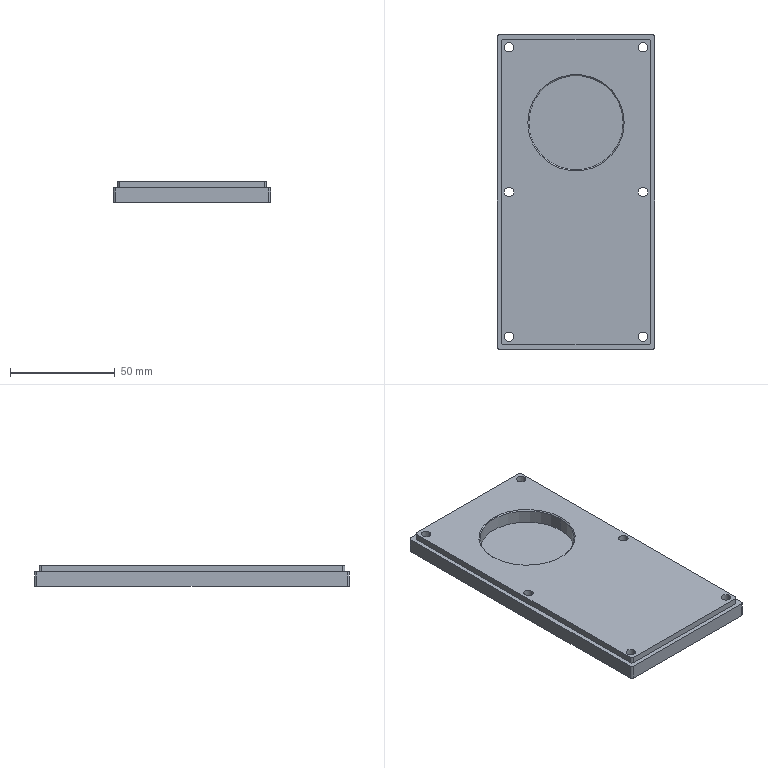Part | STEP file | 12底Plate EDA50-R-012-BZ^EDA50-R04 (D60N) | 1 solid | 54 faces | box 75 x 150 x 10 mm | volume 96841 mm3 | cylinder 34 | plane 18 | cone 2 | commonest cylinder face diameters 4.5 x12 7.5 x12 2 x8 45 x2